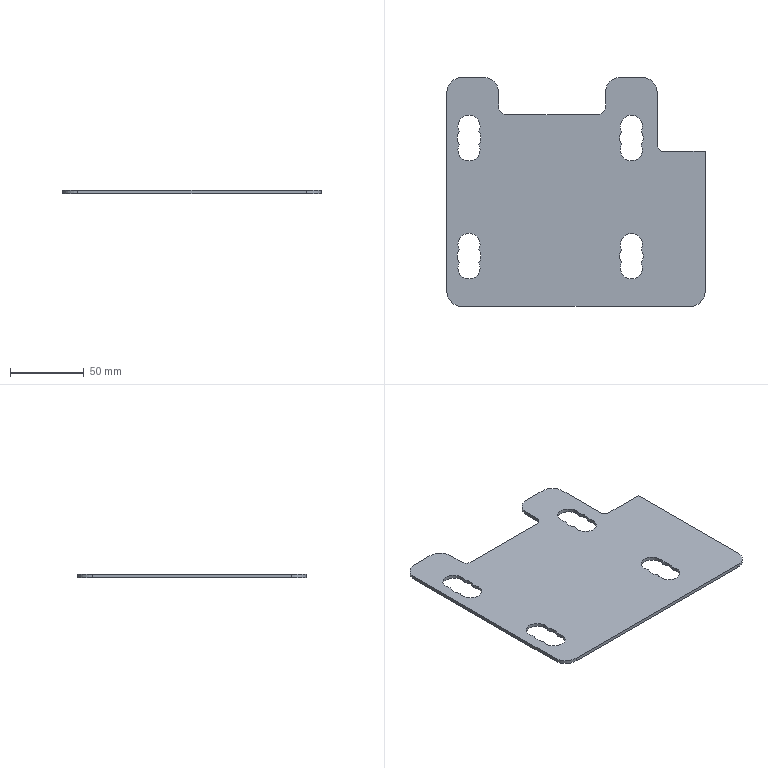Part | SolidWorks | features FlatPattern 1, SMBaseFlange 1, SheetMetal 1 | 1 solid | 57 faces | box 175 x 155 x 2.3 mm | volume 50413 mm3 | cylinder 44 | plane 13 | commonest cylinder face diameters 15 x24 16 x12 20 x6 10 x2